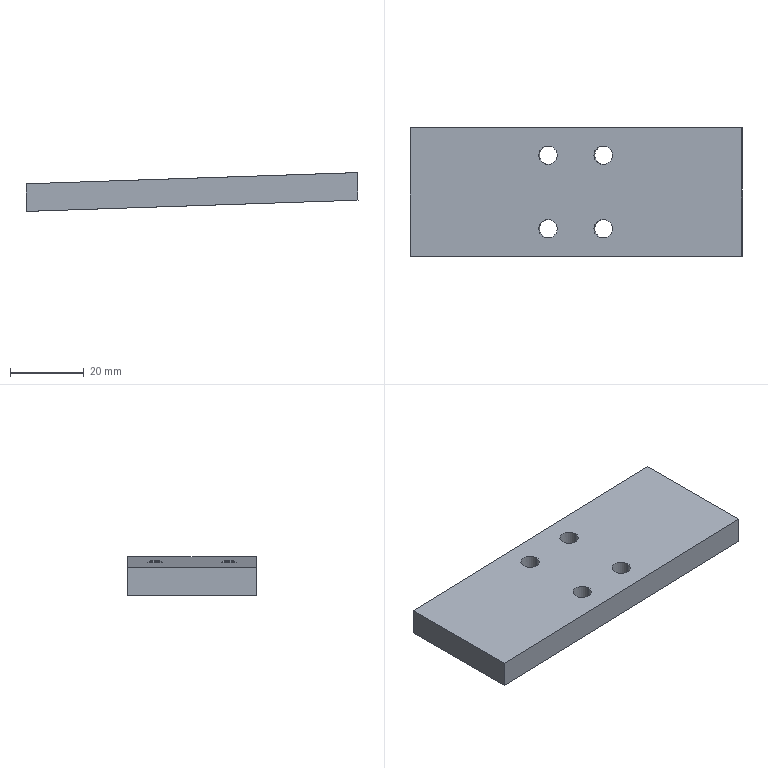Part | STEP file | 2026.6.15-Main Assembly图.sldasm-Part-154 | 1 solid | 14 faces | box 90.202 x 35 x 10.539 mm | volume 23036 mm3 | cylinder 8 | plane 6 | commonest cylinder face diameters 5 x8
STEP:
#1=CARTESIAN_POINT('',(-1600.739,658.051,4253.253));
#2=VERTEX_POINT('',#1);
#3=CARTESIAN_POINT('',(-1595.741,658.051,4253.422));
#4=VERTEX_POINT('',#3);
#5=CARTESIAN_POINT('',(-1598.24,658.051,4253.337));
#6=DIRECTION('',(-0.03381,0.,0.9994));
#7=DIRECTION('',(0.,-1.,0.));
#8=AXIS2_PLACEMENT_3D('',#5,#6,#7);
#9=CIRCLE('',#8,2.5);
#10=EDGE_CURVE('',#2,#4,#9,.T.);
#11=ORIENTED_EDGE('',*,*,#10,.F.);
#12=CARTESIAN_POINT('',(-1600.992,658.051,4260.748));
#13=VERTEX_POINT('',#12);
#14=CARTESIAN_POINT('',(-1600.739,658.051,4253.253));
#15=DIRECTION('',(-0.03381,0.,0.9994));
#16=VECTOR('',#15,1000.);
#17=LINE('',#14,#16);
#18=EDGE_CURVE('',#2,#13,#17,.T.);
#19=ORIENTED_EDGE('',*,*,#18,.T.);
#20=CARTESIAN_POINT('',(-1595.995,658.051,4260.917));
#21=VERTEX_POINT('',#20);
#22=CARTESIAN_POINT('',(-1598.494,658.051,4260.833));
#23=DIRECTION('',(-0.03381,0.,0.9994));
#24=DIRECTION('',(0.,-1.,0.));
#25=AXIS2_PLACEMENT_3D('',#22,#23,#24);
#26=CIRCLE('',#25,2.5);
#27=EDGE_CURVE('',#13,#21,#26,.T.);
#28=ORIENTED_EDGE('',*,*,#27,.T.);
#29=CARTESIAN_POINT('',(-1595.741,658.051,4253.422));
#30=DIRECTION('',(-0.03381,0.,0.9994));
#31=VECTOR('',#30,1000.);
#32=LINE('',#29,#31);
#33=EDGE_CURVE('',#4,#21,#32,.T.);
#34=ORIENTED_EDGE('',*,*,#33,.F.);
#35=EDGE_LOOP('',(#11,#19,#28,#34));
#36=FACE_OUTER_BOUND('',#35,.T.);
#37=CARTESIAN_POINT('',(-1598.24,658.051,4253.337));
#38=DIRECTION('',(-0.03381,0.,0.9994));
#39=DIRECTION('',(0.9994,0.,0.03381));
#40=AXIS2_PLACEMENT_3D('',#37,#38,#39);
#41=CYLINDRICAL_SURFACE('',#40,2.5);
#42=ADVANCED_FACE('',(#36),#41,.F.);
#43=CARTESIAN_POINT('',(-1585.747,678.051,4253.76));
#44=VERTEX_POINT('',#43);
#45=CARTESIAN_POINT('',(-1580.75,678.051,4253.929));
#46=VERTEX_POINT('',#45);
#47=CARTESIAN_POINT('',(-1583.249,678.051,4253.844));
#48=DIRECTION('',(-0.03381,0.,0.9994));
#49=DIRECTION('',(0.,-1.,0.));
#50=AXIS2_PLACEMENT_3D('',#47,#48,#49);
#51=CIRCLE('',#50,2.5);
#52=EDGE_CURVE('',#44,#46,#51,.T.);
#53=ORIENTED_EDGE('',*,*,#52,.F.);
#54=CARTESIAN_POINT('',(-1586.001,678.051,4261.256));
#55=VERTEX_POINT('',#54);
#56=CARTESIAN_POINT('',(-1585.747,678.051,4253.76));
#57=DIRECTION('',(-0.03381,0.,0.9994));
#58=VECTOR('',#57,1000.);
#59=LINE('',#56,#58);
#60=EDGE_CURVE('',#44,#55,#59,.T.);
#61=ORIENTED_EDGE('',*,*,#60,.T.);
#62=CARTESIAN_POINT('',(-1581.004,678.051,4261.425));
#63=VERTEX_POINT('',#62);
#64=CARTESIAN_POINT('',(-1583.502,678.051,4261.34));
#65=DIRECTION('',(-0.03381,0.,0.9994));
#66=DIRECTION('',(0.,-1.,0.));
#67=AXIS2_PLACEMENT_3D('',#64,#65,#66);
#68=CIRCLE('',#67,2.5);
#69=EDGE_CURVE('',#55,#63,#68,.T.);
#70=ORIENTED_EDGE('',*,*,#69,.T.);
#71=CARTESIAN_POINT('',(-1580.75,678.051,4253.929));
#72=DIRECTION('',(-0.03381,0.,0.9994));
#73=VECTOR('',#72,1000.);
#74=LINE('',#71,#73);
#75=EDGE_CURVE('',#46,#63,#74,.T.);
#76=ORIENTED_EDGE('',*,*,#75,.F.);
#77=EDGE_LOOP('',(#53,#61,#70,#76));
#78=FACE_OUTER_BOUND('',#77,.T.);
#79=CARTESIAN_POINT('',(-1583.249,678.051,4253.844));
#80=DIRECTION('',(-0.03381,0.,0.9994));
#81=DIRECTION('',(0.9994,0.,0.03381));
#82=AXIS2_PLACEMENT_3D('',#79,#80,#81);
#83=CYLINDRICAL_SURFACE('',#82,2.5);
#84=ADVANCED_FACE('',(#78),#83,.F.);
#85=CARTESIAN_POINT('',(-1585.747,658.051,4253.76));
#86=VERTEX_POINT('',#85);
#87=CARTESIAN_POINT('',(-1580.75,658.051,4253.929));
#88=VERTEX_POINT('',#87);
#89=CARTESIAN_POINT('',(-1583.249,658.051,4253.844));
#90=DIRECTION('',(-0.03381,0.,0.9994));
#91=DIRECTION('',(0.,-1.,0.));
#92=AXIS2_PLACEMENT_3D('',#89,#90,#91);
#93=CIRCLE('',#92,2.5);
#94=EDGE_CURVE('',#86,#88,#93,.T.);
#95=ORIENTED_EDGE('',*,*,#94,.F.);
#96=CARTESIAN_POINT('',(-1586.001,658.051,4261.256));
#97=VERTEX_POINT('',#96);
#98=CARTESIAN_POINT('',(-1585.747,658.051,4253.76));
#99=DIRECTION('',(-0.03381,0.,0.9994));
#100=VECTOR('',#99,1000.);
#101=LINE('',#98,#100);
#102=EDGE_CURVE('',#86,#97,#101,.T.);
#103=ORIENTED_EDGE('',*,*,#102,.T.);
#104=CARTESIAN_POINT('',(-1581.004,658.051,4261.425));
#105=VERTEX_POINT('',#104);
#106=CARTESIAN_POINT('',(-1583.502,658.051,4261.34));
#107=DIRECTION('',(-0.03381,0.,0.9994));
#108=DIRECTION('',(0.,-1.,0.));
#109=AXIS2_PLACEMENT_3D('',#106,#107,#108);
#110=CIRCLE('',#109,2.5);
#111=EDGE_CURVE('',#97,#105,#110,.T.);
#112=ORIENTED_EDGE('',*,*,#111,.T.);
#113=CARTESIAN_POINT('',(-1580.75,658.051,4253.929));
#114=DIRECTION('',(-0.03381,0.,0.9994));
#115=VECTOR('',#114,1000.);
#116=LINE('',#113,#115);
#117=EDGE_CURVE('',#88,#105,#116,.T.);
#118=ORIENTED_EDGE('',*,*,#117,.F.);
#119=EDGE_LOOP('',(#95,#103,#112,#118));
#120=FACE_OUTER_BOUND('',#119,.T.);
#121=CARTESIAN_POINT('',(-1583.249,658.051,4253.844));
#122=DIRECTION('',(-0.03381,0.,0.9994));
#123=DIRECTION('',(0.9994,0.,0.03381));
#124=AXIS2_PLACEMENT_3D('',#121,#122,#123);
#125=CYLINDRICAL_SURFACE('',#124,2.5);
#126=ADVANCED_FACE('',(#120),#125,.F.);
#127=CARTESIAN_POINT('',(-1600.739,678.051,4253.253));
#128=VERTEX_POINT('',#127);
#129=CARTESIAN_POINT('',(-1595.741,678.051,4253.422));
#130=VERTEX_POINT('',#129);
#131=CARTESIAN_POINT('',(-1598.24,678.051,4253.337));
#132=DIRECTION('',(-0.03381,0.,0.9994));
#133=DIRECTION('',(0.,-1.,0.));
#134=AXIS2_PLACEMENT_3D('',#131,#132,#133);
#135=CIRCLE('',#134,2.5);
#136=EDGE_CURVE('',#128,#130,#135,.T.);
#137=ORIENTED_EDGE('',*,*,#136,.F.);
#138=CARTESIAN_POINT('',(-1600.992,678.051,4260.748));
#139=VERTEX_POINT('',#138);
#140=CARTESIAN_POINT('',(-1600.739,678.051,4253.253));
#141=DIRECTION('',(-0.03381,0.,0.9994));
#142=VECTOR('',#141,1000.);
#143=LINE('',#140,#142);
#144=EDGE_CURVE('',#128,#139,#143,.T.);
#145=ORIENTED_EDGE('',*,*,#144,.T.);
#146=CARTESIAN_POINT('',(-1595.995,678.051,4260.917));
#147=VERTEX_POINT('',#146);
#148=CARTESIAN_POINT('',(-1598.494,678.051,4260.833));
#149=DIRECTION('',(-0.03381,0.,0.9994));
#150=DIRECTION('',(0.,-1.,0.));
#151=AXIS2_PLACEMENT_3D('',#148,#149,#150);
#152=CIRCLE('',#151,2.5);
#153=EDGE_CURVE('',#139,#147,#152,.T.);
#154=ORIENTED_EDGE('',*,*,#153,.T.);
#155=CARTESIAN_POINT('',(-1595.741,678.051,4253.422));
#156=DIRECTION('',(-0.03381,0.,0.9994));
#157=VECTOR('',#156,1000.);
#158=LINE('',#155,#157);
#159=EDGE_CURVE('',#130,#147,#158,.T.);
#160=ORIENTED_EDGE('',*,*,#159,.F.);
#161=EDGE_LOOP('',(#137,#145,#154,#160));
#162=FACE_OUTER_BOUND('',#161,.T.);
#163=CARTESIAN_POINT('',(-1598.24,678.051,4253.337));
#164=DIRECTION('',(-0.03381,0.,0.9994));
#165=DIRECTION('',(0.9994,0.,0.03381));
#166=AXIS2_PLACEMENT_3D('',#163,#164,#165);
#167=CYLINDRICAL_SURFACE('',#166,2.5);
#168=ADVANCED_FACE('',(#162),#167,.F.);
#169=CARTESIAN_POINT('',(-1635.972,650.551,4259.565));
#170=VERTEX_POINT('',#169);
#171=CARTESIAN_POINT('',(-1635.972,685.551,4259.565));
#172=VERTEX_POINT('',#171);
#173=CARTESIAN_POINT('',(-1635.972,650.551,4259.565));
#174=DIRECTION('',(0.,1.,0.));
#175=VECTOR('',#174,1000.);
#176=LINE('',#173,#175);
#177=EDGE_CURVE('',#170,#172,#176,.T.);
#178=ORIENTED_EDGE('',*,*,#177,.T.);
#179=CARTESIAN_POINT('',(-1635.719,685.551,4252.069));
#180=VERTEX_POINT('',#179);
#181=CARTESIAN_POINT('',(-1635.719,685.551,4252.069));
#182=DIRECTION('',(-0.03381,0.,0.9994));
#183=VECTOR('',#182,1000.);
#184=LINE('',#181,#183);
#185=EDGE_CURVE('',#180,#172,#184,.T.);
#186=ORIENTED_EDGE('',*,*,#185,.F.);
#187=CARTESIAN_POINT('',(-1635.719,650.551,4252.069));
#188=VERTEX_POINT('',#187);
#189=CARTESIAN_POINT('',(-1635.719,650.551,4252.069));
#190=DIRECTION('',(0.,1.,0.));
#191=VECTOR('',#190,1000.);
#192=LINE('',#189,#191);
#193=EDGE_CURVE('',#188,#180,#192,.T.);
#194=ORIENTED_EDGE('',*,*,#193,.F.);
#195=CARTESIAN_POINT('',(-1635.719,650.551,4252.069));
#196=DIRECTION('',(-0.03381,0.,0.9994));
#197=VECTOR('',#196,1000.);
#198=LINE('',#195,#197);
#199=EDGE_CURVE('',#188,#170,#198,.T.);
#200=ORIENTED_EDGE('',*,*,#199,.T.);
#201=EDGE_LOOP('',(#178,#186,#194,#200));
#202=FACE_OUTER_BOUND('',#201,.T.);
#203=CARTESIAN_POINT('',(-1635.719,650.551,4252.069));
#204=DIRECTION('',(0.9994,0.,0.03381));
#205=DIRECTION('',(0.03381,0.,-0.9994));
#206=AXIS2_PLACEMENT_3D('',#203,#204,#205);
#207=PLANE('',#206);
#208=ADVANCED_FACE('',(#202),#207,.F.);
#209=CARTESIAN_POINT('',(-1546.024,685.551,4262.608));
#210=VERTEX_POINT('',#209);
#211=CARTESIAN_POINT('',(-1635.972,685.551,4259.565));
#212=DIRECTION('',(0.9994,0.,0.03381));
#213=VECTOR('',#212,1000.);
#214=LINE('',#211,#213);
#215=EDGE_CURVE('',#172,#210,#214,.T.);
#216=ORIENTED_EDGE('',*,*,#215,.T.);
#217=CARTESIAN_POINT('',(-1545.77,685.551,4255.112));
#218=VERTEX_POINT('',#217);
#219=CARTESIAN_POINT('',(-1545.77,685.551,4255.112));
#220=DIRECTION('',(-0.03381,0.,0.9994));
#221=VECTOR('',#220,1000.);
#222=LINE('',#219,#221);
#223=EDGE_CURVE('',#218,#210,#222,.T.);
#224=ORIENTED_EDGE('',*,*,#223,.F.);
#225=CARTESIAN_POINT('',(-1635.719,685.551,4252.069));
#226=DIRECTION('',(0.9994,0.,0.03381));
#227=VECTOR('',#226,1000.);
#228=LINE('',#225,#227);
#229=EDGE_CURVE('',#180,#218,#228,.T.);
#230=ORIENTED_EDGE('',*,*,#229,.F.);
#231=ORIENTED_EDGE('',*,*,#185,.T.);
#232=EDGE_LOOP('',(#216,#224,#230,#231));
#233=FACE_OUTER_BOUND('',#232,.T.);
#234=CARTESIAN_POINT('',(-1635.719,685.551,4252.069));
#235=DIRECTION('',(0.,-1.,0.));
#236=DIRECTION('',(0.,0.,-1.));
#237=AXIS2_PLACEMENT_3D('',#234,#235,#236);
#238=PLANE('',#237);
#239=ADVANCED_FACE('',(#233),#238,.F.);
#240=CARTESIAN_POINT('',(-1546.024,650.551,4262.608));
#241=VERTEX_POINT('',#240);
#242=CARTESIAN_POINT('',(-1546.024,685.551,4262.608));
#243=DIRECTION('',(0.,-1.,0.));
#244=VECTOR('',#243,1000.);
#245=LINE('',#242,#244);
#246=EDGE_CURVE('',#210,#241,#245,.T.);
#247=ORIENTED_EDGE('',*,*,#246,.T.);
#248=CARTESIAN_POINT('',(-1545.77,650.551,4255.112));
#249=VERTEX_POINT('',#248);
#250=CARTESIAN_POINT('',(-1545.77,650.551,4255.112));
#251=DIRECTION('',(-0.03381,0.,0.9994));
#252=VECTOR('',#251,1000.);
#253=LINE('',#250,#252);
#254=EDGE_CURVE('',#249,#241,#253,.T.);
#255=ORIENTED_EDGE('',*,*,#254,.F.);
#256=CARTESIAN_POINT('',(-1545.77,685.551,4255.112));
#257=DIRECTION('',(0.,-1.,0.));
#258=VECTOR('',#257,1000.);
#259=LINE('',#256,#258);
#260=EDGE_CURVE('',#218,#249,#259,.T.);
#261=ORIENTED_EDGE('',*,*,#260,.F.);
#262=ORIENTED_EDGE('',*,*,#223,.T.);
#263=EDGE_LOOP('',(#247,#255,#261,#262));
#264=FACE_OUTER_BOUND('',#263,.T.);
#265=CARTESIAN_POINT('',(-1545.77,685.551,4255.112));
#266=DIRECTION('',(-0.9994,0.,-0.03381));
#267=DIRECTION('',(-0.03381,0.,0.9994));
#268=AXIS2_PLACEMENT_3D('',#265,#266,#267);
#269=PLANE('',#268);
#270=ADVANCED_FACE('',(#264),#269,.F.);
#271=ORIENTED_EDGE('',*,*,#144,.F.);
#272=CARTESIAN_POINT('',(-1598.24,678.051,4253.337));
#273=DIRECTION('',(-0.03381,0.,0.9994));
#274=DIRECTION('',(0.,-1.,0.));
#275=AXIS2_PLACEMENT_3D('',#272,#273,#274);
#276=CIRCLE('',#275,2.5);
#277=EDGE_CURVE('',#130,#128,#276,.T.);
#278=ORIENTED_EDGE('',*,*,#277,.F.);
#279=ORIENTED_EDGE('',*,*,#159,.T.);
#280=CARTESIAN_POINT('',(-1598.494,678.051,4260.833));
#281=DIRECTION('',(-0.03381,0.,0.9994));
#282=DIRECTION('',(0.,-1.,0.));
#283=AXIS2_PLACEMENT_3D('',#280,#281,#282);
#284=CIRCLE('',#283,2.5);
#285=EDGE_CURVE('',#147,#139,#284,.T.);
#286=ORIENTED_EDGE('',*,*,#285,.T.);
#287=EDGE_LOOP('',(#271,#278,#279,#286));
#288=FACE_OUTER_BOUND('',#287,.T.);
#289=CARTESIAN_POINT('',(-1598.24,678.051,4253.337));
#290=DIRECTION('',(-0.03381,0.,0.9994));
#291=DIRECTION('',(0.9994,0.,0.03381));
#292=AXIS2_PLACEMENT_3D('',#289,#290,#291);
#293=CYLINDRICAL_SURFACE('',#292,2.5);
#294=ADVANCED_FACE('',(#288),#293,.F.);
#295=ORIENTED_EDGE('',*,*,#102,.F.);
#296=CARTESIAN_POINT('',(-1583.249,658.051,4253.844));
#297=DIRECTION('',(-0.03381,0.,0.9994));
#298=DIRECTION('',(0.,-1.,0.));
#299=AXIS2_PLACEMENT_3D('',#296,#297,#298);
#300=CIRCLE('',#299,2.5);
#301=EDGE_CURVE('',#88,#86,#300,.T.);
#302=ORIENTED_EDGE('',*,*,#301,.F.);
#303=ORIENTED_EDGE('',*,*,#117,.T.);
#304=CARTESIAN_POINT('',(-1583.502,658.051,4261.34));
#305=DIRECTION('',(-0.03381,0.,0.9994));
#306=DIRECTION('',(0.,-1.,0.));
#307=AXIS2_PLACEMENT_3D('',#304,#305,#306);
#308=CIRCLE('',#307,2.5);
#309=EDGE_CURVE('',#105,#97,#308,.T.);
#310=ORIENTED_EDGE('',*,*,#309,.T.);
#311=EDGE_LOOP('',(#295,#302,#303,#310));
#312=FACE_OUTER_BOUND('',#311,.T.);
#313=CARTESIAN_POINT('',(-1583.249,658.051,4253.844));
#314=DIRECTION('',(-0.03381,0.,0.9994));
#315=DIRECTION('',(0.9994,0.,0.03381));
#316=AXIS2_PLACEMENT_3D('',#313,#314,#315);
#317=CYLINDRICAL_SURFACE('',#316,2.5);
#318=ADVANCED_FACE('',(#312),#317,.F.);
#319=ORIENTED_EDGE('',*,*,#60,.F.);
#320=CARTESIAN_POINT('',(-1583.249,678.051,4253.844));
#321=DIRECTION('',(-0.03381,0.,0.9994));
#322=DIRECTION('',(0.,-1.,0.));
#323=AXIS2_PLACEMENT_3D('',#320,#321,#322);
#324=CIRCLE('',#323,2.5);
#325=EDGE_CURVE('',#46,#44,#324,.T.);
#326=ORIENTED_EDGE('',*,*,#325,.F.);
#327=ORIENTED_EDGE('',*,*,#75,.T.);
#328=CARTESIAN_POINT('',(-1583.502,678.051,4261.34));
#329=DIRECTION('',(-0.03381,0.,0.9994));
#330=DIRECTION('',(0.,-1.,0.));
#331=AXIS2_PLACEMENT_3D('',#328,#329,#330);
#332=CIRCLE('',#331,2.5);
#333=EDGE_CURVE('',#63,#55,#332,.T.);
#334=ORIENTED_EDGE('',*,*,#333,.T.);
#335=EDGE_LOOP('',(#319,#326,#327,#334));
#336=FACE_OUTER_BOUND('',#335,.T.);
#337=CARTESIAN_POINT('',(-1583.249,678.051,4253.844));
#338=DIRECTION('',(-0.03381,0.,0.9994));
#339=DIRECTION('',(0.9994,0.,0.03381));
#340=AXIS2_PLACEMENT_3D('',#337,#338,#339);
#341=CYLINDRICAL_SURFACE('',#340,2.5);
#342=ADVANCED_FACE('',(#336),#341,.F.);
#343=CARTESIAN_POINT('',(-1546.024,650.551,4262.608));
#344=DIRECTION('',(-0.9994,0.,-0.03381));
#345=VECTOR('',#344,1000.);
#346=LINE('',#343,#345);
#347=EDGE_CURVE('',#241,#170,#346,.T.);
#348=ORIENTED_EDGE('',*,*,#347,.T.);
#349=ORIENTED_EDGE('',*,*,#199,.F.);
#350=CARTESIAN_POINT('',(-1545.77,650.551,4255.112));
#351=DIRECTION('',(-0.9994,0.,-0.03381));
#352=VECTOR('',#351,1000.);
#353=LINE('',#350,#352);
#354=EDGE_CURVE('',#249,#188,#353,.T.);
#355=ORIENTED_EDGE('',*,*,#354,.F.);
#356=ORIENTED_EDGE('',*,*,#254,.T.);
#357=EDGE_LOOP('',(#348,#349,#355,#356));
#358=FACE_OUTER_BOUND('',#357,.T.);
#359=CARTESIAN_POINT('',(-1545.77,650.551,4255.112));
#360=DIRECTION('',(0.,1.,0.));
#361=DIRECTION('',(0.,0.,1.));
#362=AXIS2_PLACEMENT_3D('',#359,#360,#361);
#363=PLANE('',#362);
#364=ADVANCED_FACE('',(#358),#363,.F.);
#365=ORIENTED_EDGE('',*,*,#18,.F.);
#366=CARTESIAN_POINT('',(-1598.24,658.051,4253.337));
#367=DIRECTION('',(-0.03381,0.,0.9994));
#368=DIRECTION('',(0.,-1.,0.));
#369=AXIS2_PLACEMENT_3D('',#366,#367,#368);
#370=CIRCLE('',#369,2.5);
#371=EDGE_CURVE('',#4,#2,#370,.T.);
#372=ORIENTED_EDGE('',*,*,#371,.F.);
#373=ORIENTED_EDGE('',*,*,#33,.T.);
#374=CARTESIAN_POINT('',(-1598.494,658.051,4260.833));
#375=DIRECTION('',(-0.03381,0.,0.9994));
#376=DIRECTION('',(0.,-1.,0.));
#377=AXIS2_PLACEMENT_3D('',#374,#375,#376);
#378=CIRCLE('',#377,2.5);
#379=EDGE_CURVE('',#21,#13,#378,.T.);
#380=ORIENTED_EDGE('',*,*,#379,.T.);
#381=EDGE_LOOP('',(#365,#372,#373,#380));
#382=FACE_OUTER_BOUND('',#381,.T.);
#383=CARTESIAN_POINT('',(-1598.24,658.051,4253.337));
#384=DIRECTION('',(-0.03381,0.,0.9994));
#385=DIRECTION('',(0.9994,0.,0.03381));
#386=AXIS2_PLACEMENT_3D('',#383,#384,#385);
#387=CYLINDRICAL_SURFACE('',#386,2.5);
#388=ADVANCED_FACE('',(#382),#387,.F.);
#389=ORIENTED_EDGE('',*,*,#193,.T.);
#390=ORIENTED_EDGE('',*,*,#229,.T.);
#391=ORIENTED_EDGE('',*,*,#260,.T.);
#392=ORIENTED_EDGE('',*,*,#354,.T.);
#393=EDGE_LOOP('',(#389,#390,#391,#392));
#394=FACE_OUTER_BOUND('',#393,.T.);
#395=ORIENTED_EDGE('',*,*,#325,.T.);
#396=ORIENTED_EDGE('',*,*,#52,.T.);
#397=EDGE_LOOP('',(#395,#396));
#398=FACE_BOUND('',#397,.T.);
#399=ORIENTED_EDGE('',*,*,#301,.T.);
#400=ORIENTED_EDGE('',*,*,#94,.T.);
#401=EDGE_LOOP('',(#399,#400));
#402=FACE_BOUND('',#401,.T.);
#403=ORIENTED_EDGE('',*,*,#277,.T.);
#404=ORIENTED_EDGE('',*,*,#136,.T.);
#405=EDGE_LOOP('',(#403,#404));
#406=FACE_BOUND('',#405,.T.);
#407=ORIENTED_EDGE('',*,*,#371,.T.);
#408=ORIENTED_EDGE('',*,*,#10,.T.);
#409=EDGE_LOOP('',(#407,#408));
#410=FACE_BOUND('',#409,.T.);
#411=CARTESIAN_POINT('',(-1583.249,678.051,4253.844));
#412=DIRECTION('',(-0.03381,0.,0.9994));
#413=DIRECTION('',(0.9994,0.,0.03381));
#414=AXIS2_PLACEMENT_3D('',#411,#412,#413);
#415=PLANE('',#414);
#416=ADVANCED_FACE('',(#394,#398,#402,#406,#410),#415,.F.);
#417=ORIENTED_EDGE('',*,*,#177,.F.);
#418=ORIENTED_EDGE('',*,*,#347,.F.);
#419=ORIENTED_EDGE('',*,*,#246,.F.);
#420=ORIENTED_EDGE('',*,*,#215,.F.);
#421=EDGE_LOOP('',(#417,#418,#419,#420));
#422=FACE_OUTER_BOUND('',#421,.T.);
#423=ORIENTED_EDGE('',*,*,#333,.F.);
#424=ORIENTED_EDGE('',*,*,#69,.F.);
#425=EDGE_LOOP('',(#423,#424));
#426=FACE_BOUND('',#425,.T.);
#427=ORIENTED_EDGE('',*,*,#309,.F.);
#428=ORIENTED_EDGE('',*,*,#111,.F.);
#429=EDGE_LOOP('',(#427,#428));
#430=FACE_BOUND('',#429,.T.);
#431=ORIENTED_EDGE('',*,*,#285,.F.);
#432=ORIENTED_EDGE('',*,*,#153,.F.);
#433=EDGE_LOOP('',(#431,#432));
#434=FACE_BOUND('',#433,.T.);
#435=ORIENTED_EDGE('',*,*,#379,.F.);
#436=ORIENTED_EDGE('',*,*,#27,.F.);
#437=EDGE_LOOP('',(#435,#436));
#438=FACE_BOUND('',#437,.T.);
#439=CARTESIAN_POINT('',(-1583.502,678.051,4261.34));
#440=DIRECTION('',(-0.03381,0.,0.9994));
#441=DIRECTION('',(0.9994,0.,0.03381));
#442=AXIS2_PLACEMENT_3D('',#439,#440,#441);
#443=PLANE('',#442);
#444=ADVANCED_FACE('',(#422,#426,#430,#434,#438),#443,.T.);
#445=CLOSED_SHELL('',(#42,#84,#126,#168,#208,#239,#270,#294,#318,#342,#364,#388,#416,#444));
#446=MANIFOLD_SOLID_BREP('',#445);
#447=CARTESIAN_POINT('',(0.,0.,0.));
#448=DIRECTION('',(0.,0.,1.));
#449=DIRECTION('',(1.,0.,0.));
#450=AXIS2_PLACEMENT_3D('',#447,#448,#449);
#451=(LENGTH_UNIT()NAMED_UNIT(*)SI_UNIT(.MILLI.,.METRE.));
#452=UNCERTAINTY_MEASURE_WITH_UNIT(LENGTH_MEASURE(0.00001),#451,'','');
#453=(NAMED_UNIT(*)PLANE_ANGLE_UNIT()SI_UNIT($,.RADIAN.));
#454=(NAMED_UNIT(*)SI_UNIT($,.STERADIAN.)SOLID_ANGLE_UNIT());
#455=(GEOMETRIC_REPRESENTATION_CONTEXT(3)GLOBAL_UNCERTAINTY_ASSIGNED_CONTEXT((#452))GLOBAL_UNIT_ASSIGNED_CONTEXT((#451,#453,#454))REPRESENTATION_CONTEXT('',''));
#456=ADVANCED_BREP_SHAPE_REPRESENTATION('',(#446,#450),#455);